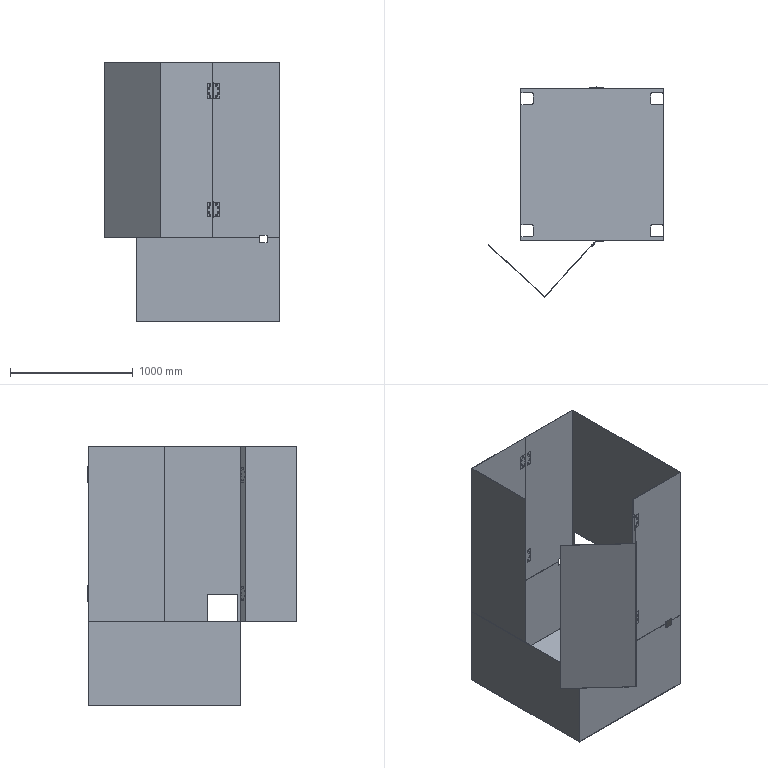Part | SolidWorks | features CompositeCurve 2 | 16 solids | 488 faces | box 1424 x 1708 x 2109 mm | volume 23017805 mm3 | cylinder 228 | plane 180 | cone 64 | sphere 16 | commonest cylinder face diameters 8.5 x64 9 x64 7 x40 10 x36 20 x16 6.5 x8